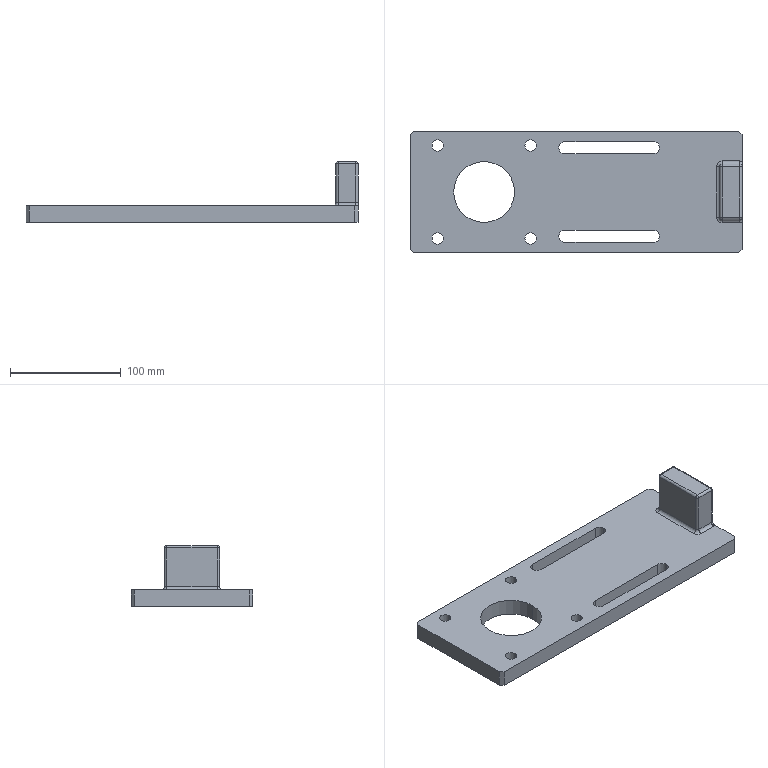Part | STEP file | Adjusting plate-1XG | 1 solid | 53 faces | box 300 x 110 x 55 mm | volume 464863 mm3 | cylinder 27 | plane 18 | torus 4 | sphere 4 | commonest cylinder face diameters 4 x8 10.2 x8 11 x6 6 x3 55 x2